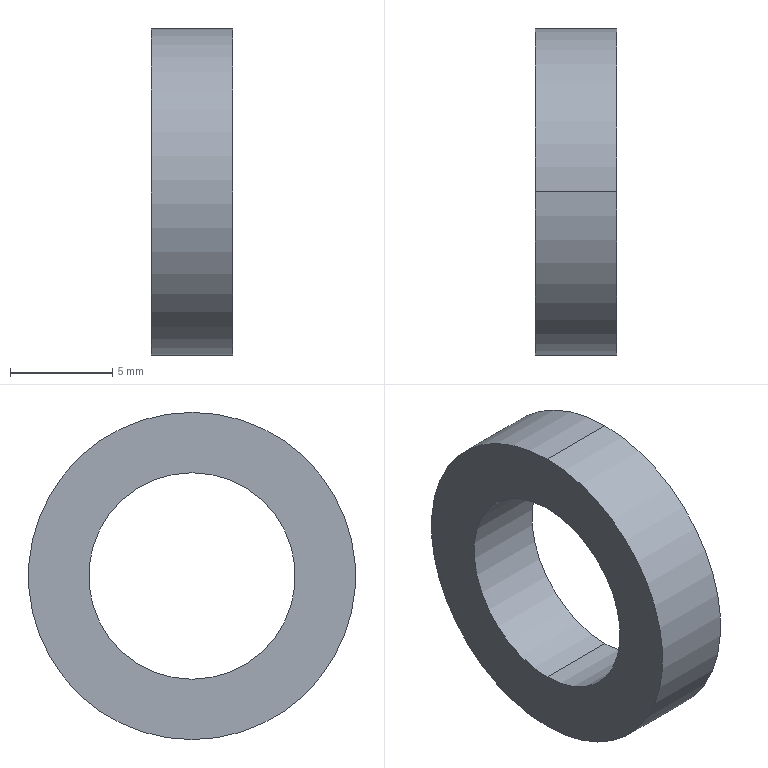Part | SolidWorks | features BaseBody 1 | 1 solid | 6 faces | box 4 x 16 x 16 mm | volume 483.774 mm3 | cylinder 4 | plane 2 | commonest cylinder face diameters 10.1 x2 16 x2
STEP:
#1=CARTESIAN_POINT('',(-2.,0.,-8.));
#2=VERTEX_POINT('',#1);
#3=CARTESIAN_POINT('',(-2.,0.,8.));
#4=VERTEX_POINT('',#3);
#5=CARTESIAN_POINT('',(-2.,0.,0.));
#6=DIRECTION('',(1.,0.,0.));
#7=DIRECTION('',(0.,0.,-1.));
#8=AXIS2_PLACEMENT_3D('',#5,#6,#7);
#9=CIRCLE('',#8,8.);
#10=EDGE_CURVE('',#2,#4,#9,.T.);
#11=ORIENTED_EDGE('',*,*,#10,.T.);
#12=CARTESIAN_POINT('',(2.,0.,8.));
#13=VERTEX_POINT('',#12);
#14=CARTESIAN_POINT('',(-2.,0.,8.));
#15=DIRECTION('',(1.,0.,0.));
#16=VECTOR('',#15,1000.);
#17=LINE('',#14,#16);
#18=EDGE_CURVE('',#4,#13,#17,.T.);
#19=ORIENTED_EDGE('',*,*,#18,.T.);
#20=CARTESIAN_POINT('',(2.,0.,-8.));
#21=VERTEX_POINT('',#20);
#22=CARTESIAN_POINT('',(2.,0.,0.));
#23=DIRECTION('',(-1.,0.,0.));
#24=DIRECTION('',(0.,0.,-1.));
#25=AXIS2_PLACEMENT_3D('',#22,#23,#24);
#26=CIRCLE('',#25,8.);
#27=EDGE_CURVE('',#13,#21,#26,.T.);
#28=ORIENTED_EDGE('',*,*,#27,.T.);
#29=CARTESIAN_POINT('',(-2.,0.,-8.));
#30=DIRECTION('',(1.,0.,0.));
#31=VECTOR('',#30,1000.);
#32=LINE('',#29,#31);
#33=EDGE_CURVE('',#2,#21,#32,.T.);
#34=ORIENTED_EDGE('',*,*,#33,.F.);
#35=EDGE_LOOP('',(#11,#19,#28,#34));
#36=FACE_OUTER_BOUND('',#35,.T.);
#37=CARTESIAN_POINT('',(-2.,0.,0.));
#38=DIRECTION('',(1.,0.,0.));
#39=DIRECTION('',(0.,0.,-1.));
#40=AXIS2_PLACEMENT_3D('',#37,#38,#39);
#41=CYLINDRICAL_SURFACE('',#40,8.);
#42=ADVANCED_FACE('',(#36),#41,.T.);
#43=CARTESIAN_POINT('',(-2.,0.,-5.05));
#44=VERTEX_POINT('',#43);
#45=CARTESIAN_POINT('',(-2.,0.,5.05));
#46=VERTEX_POINT('',#45);
#47=CARTESIAN_POINT('',(-2.,0.,0.));
#48=DIRECTION('',(-1.,0.,0.));
#49=DIRECTION('',(0.,0.,-1.));
#50=AXIS2_PLACEMENT_3D('',#47,#48,#49);
#51=CIRCLE('',#50,5.05);
#52=EDGE_CURVE('',#44,#46,#51,.T.);
#53=ORIENTED_EDGE('',*,*,#52,.T.);
#54=CARTESIAN_POINT('',(2.,0.,5.05));
#55=VERTEX_POINT('',#54);
#56=CARTESIAN_POINT('',(-3.,0.,5.05));
#57=DIRECTION('',(1.,0.,0.));
#58=VECTOR('',#57,1000.);
#59=LINE('',#56,#58);
#60=EDGE_CURVE('',#46,#55,#59,.T.);
#61=ORIENTED_EDGE('',*,*,#60,.T.);
#62=CARTESIAN_POINT('',(2.,0.,-5.05));
#63=VERTEX_POINT('',#62);
#64=CARTESIAN_POINT('',(2.,0.,0.));
#65=DIRECTION('',(-1.,0.,0.));
#66=DIRECTION('',(0.,0.,-1.));
#67=AXIS2_PLACEMENT_3D('',#64,#65,#66);
#68=CIRCLE('',#67,5.05);
#69=EDGE_CURVE('',#63,#55,#68,.T.);
#70=ORIENTED_EDGE('',*,*,#69,.F.);
#71=CARTESIAN_POINT('',(-3.,0.,-5.05));
#72=DIRECTION('',(1.,0.,0.));
#73=VECTOR('',#72,1000.);
#74=LINE('',#71,#73);
#75=EDGE_CURVE('',#44,#63,#74,.T.);
#76=ORIENTED_EDGE('',*,*,#75,.F.);
#77=EDGE_LOOP('',(#53,#61,#70,#76));
#78=FACE_OUTER_BOUND('',#77,.T.);
#79=CARTESIAN_POINT('',(-3.,0.,0.));
#80=DIRECTION('',(1.,0.,0.));
#81=DIRECTION('',(0.,0.,-1.));
#82=AXIS2_PLACEMENT_3D('',#79,#80,#81);
#83=CYLINDRICAL_SURFACE('',#82,5.05);
#84=ADVANCED_FACE('',(#78),#83,.F.);
#85=ORIENTED_EDGE('',*,*,#18,.F.);
#86=CARTESIAN_POINT('',(-2.,0.,0.));
#87=DIRECTION('',(1.,0.,0.));
#88=DIRECTION('',(0.,0.,-1.));
#89=AXIS2_PLACEMENT_3D('',#86,#87,#88);
#90=CIRCLE('',#89,8.);
#91=EDGE_CURVE('',#4,#2,#90,.T.);
#92=ORIENTED_EDGE('',*,*,#91,.T.);
#93=ORIENTED_EDGE('',*,*,#33,.T.);
#94=CARTESIAN_POINT('',(2.,0.,0.));
#95=DIRECTION('',(-1.,0.,0.));
#96=DIRECTION('',(0.,0.,-1.));
#97=AXIS2_PLACEMENT_3D('',#94,#95,#96);
#98=CIRCLE('',#97,8.);
#99=EDGE_CURVE('',#21,#13,#98,.T.);
#100=ORIENTED_EDGE('',*,*,#99,.T.);
#101=EDGE_LOOP('',(#85,#92,#93,#100));
#102=FACE_OUTER_BOUND('',#101,.T.);
#103=CARTESIAN_POINT('',(-2.,0.,0.));
#104=DIRECTION('',(1.,0.,0.));
#105=DIRECTION('',(0.,0.,-1.));
#106=AXIS2_PLACEMENT_3D('',#103,#104,#105);
#107=CYLINDRICAL_SURFACE('',#106,8.);
#108=ADVANCED_FACE('',(#102),#107,.T.);
#109=ORIENTED_EDGE('',*,*,#52,.F.);
#110=CARTESIAN_POINT('',(-2.,0.,0.));
#111=DIRECTION('',(-1.,0.,0.));
#112=DIRECTION('',(0.,0.,-1.));
#113=AXIS2_PLACEMENT_3D('',#110,#111,#112);
#114=CIRCLE('',#113,5.05);
#115=EDGE_CURVE('',#46,#44,#114,.T.);
#116=ORIENTED_EDGE('',*,*,#115,.F.);
#117=EDGE_LOOP('',(#109,#116));
#118=FACE_BOUND('',#117,.T.);
#119=ORIENTED_EDGE('',*,*,#10,.F.);
#120=ORIENTED_EDGE('',*,*,#91,.F.);
#121=EDGE_LOOP('',(#119,#120));
#122=FACE_OUTER_BOUND('',#121,.T.);
#123=CARTESIAN_POINT('',(-2.,0.,0.));
#124=DIRECTION('',(1.,0.,0.));
#125=DIRECTION('',(0.,0.,-1.));
#126=AXIS2_PLACEMENT_3D('',#123,#124,#125);
#127=PLANE('',#126);
#128=ADVANCED_FACE('',(#118,#122),#127,.F.);
#129=ORIENTED_EDGE('',*,*,#69,.T.);
#130=CARTESIAN_POINT('',(2.,0.,0.));
#131=DIRECTION('',(-1.,0.,0.));
#132=DIRECTION('',(0.,0.,-1.));
#133=AXIS2_PLACEMENT_3D('',#130,#131,#132);
#134=CIRCLE('',#133,5.05);
#135=EDGE_CURVE('',#55,#63,#134,.T.);
#136=ORIENTED_EDGE('',*,*,#135,.T.);
#137=EDGE_LOOP('',(#129,#136));
#138=FACE_BOUND('',#137,.T.);
#139=ORIENTED_EDGE('',*,*,#99,.F.);
#140=ORIENTED_EDGE('',*,*,#27,.F.);
#141=EDGE_LOOP('',(#139,#140));
#142=FACE_OUTER_BOUND('',#141,.T.);
#143=CARTESIAN_POINT('',(2.,0.,0.));
#144=DIRECTION('',(1.,0.,0.));
#145=DIRECTION('',(0.,0.,-1.));
#146=AXIS2_PLACEMENT_3D('',#143,#144,#145);
#147=PLANE('',#146);
#148=ADVANCED_FACE('',(#138,#142),#147,.T.);
#149=ORIENTED_EDGE('',*,*,#60,.F.);
#150=ORIENTED_EDGE('',*,*,#115,.T.);
#151=ORIENTED_EDGE('',*,*,#75,.T.);
#152=ORIENTED_EDGE('',*,*,#135,.F.);
#153=EDGE_LOOP('',(#149,#150,#151,#152));
#154=FACE_OUTER_BOUND('',#153,.T.);
#155=CARTESIAN_POINT('',(-3.,0.,0.));
#156=DIRECTION('',(1.,0.,0.));
#157=DIRECTION('',(0.,0.,-1.));
#158=AXIS2_PLACEMENT_3D('',#155,#156,#157);
#159=CYLINDRICAL_SURFACE('',#158,5.05);
#160=ADVANCED_FACE('',(#154),#159,.F.);
#161=CLOSED_SHELL('',(#42,#84,#108,#128,#148,#160));
#162=MANIFOLD_SOLID_BREP('',#161);
#163=CARTESIAN_POINT('',(0.,0.,0.));
#164=DIRECTION('',(0.,0.,1.));
#165=DIRECTION('',(1.,0.,0.));
#166=AXIS2_PLACEMENT_3D('',#163,#164,#165);
#167=(LENGTH_UNIT()NAMED_UNIT(*)SI_UNIT(.MILLI.,.METRE.));
#168=UNCERTAINTY_MEASURE_WITH_UNIT(LENGTH_MEASURE(0.00001),#167,'','');
#169=(NAMED_UNIT(*)PLANE_ANGLE_UNIT()SI_UNIT($,.RADIAN.));
#170=(NAMED_UNIT(*)SI_UNIT($,.STERADIAN.)SOLID_ANGLE_UNIT());
#171=(GEOMETRIC_REPRESENTATION_CONTEXT(3)GLOBAL_UNCERTAINTY_ASSIGNED_CONTEXT((#168))GLOBAL_UNIT_ASSIGNED_CONTEXT((#167,#169,#170))REPRESENTATION_CONTEXT('',''));
#172=ADVANCED_BREP_SHAPE_REPRESENTATION('',(#162,#166),#171);